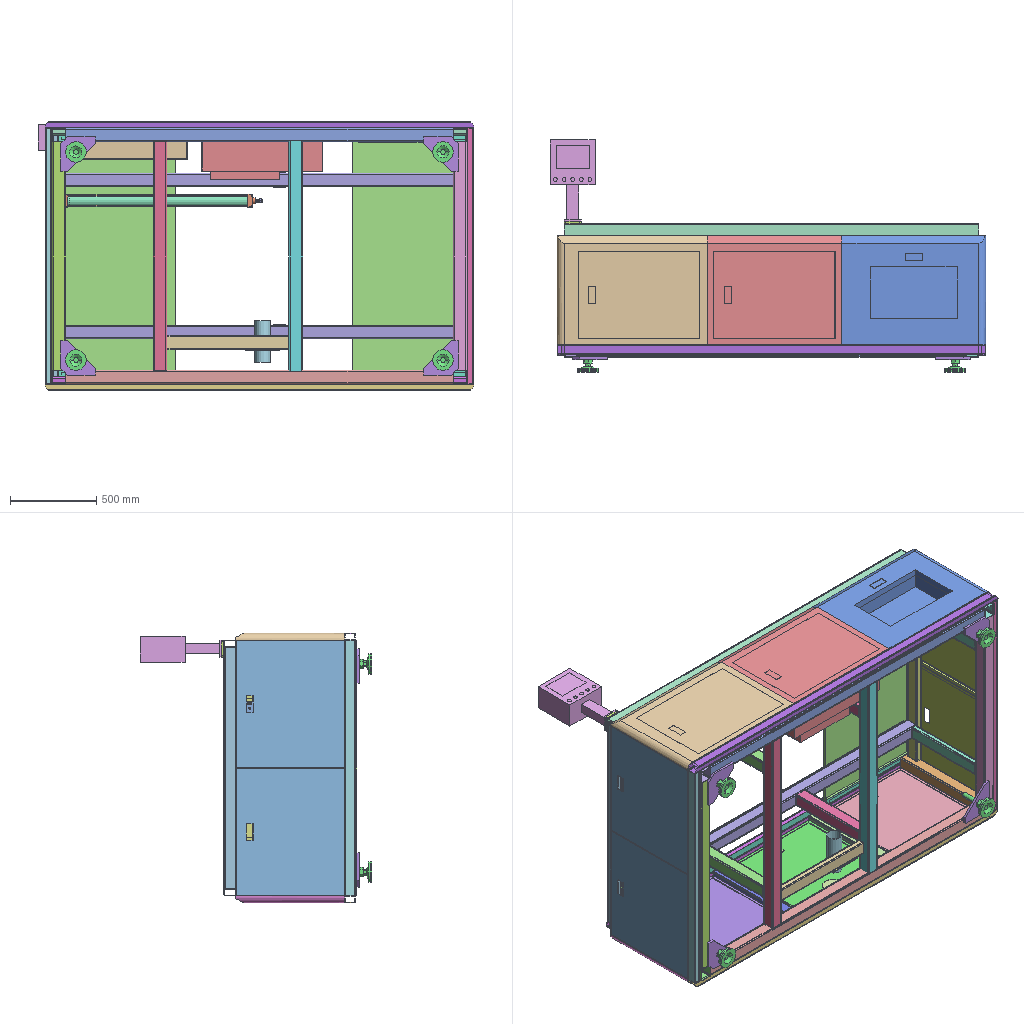Assembly | SolidWorks | 34 different items | 53 placed | box 2520 x 1341 x 1560 mm
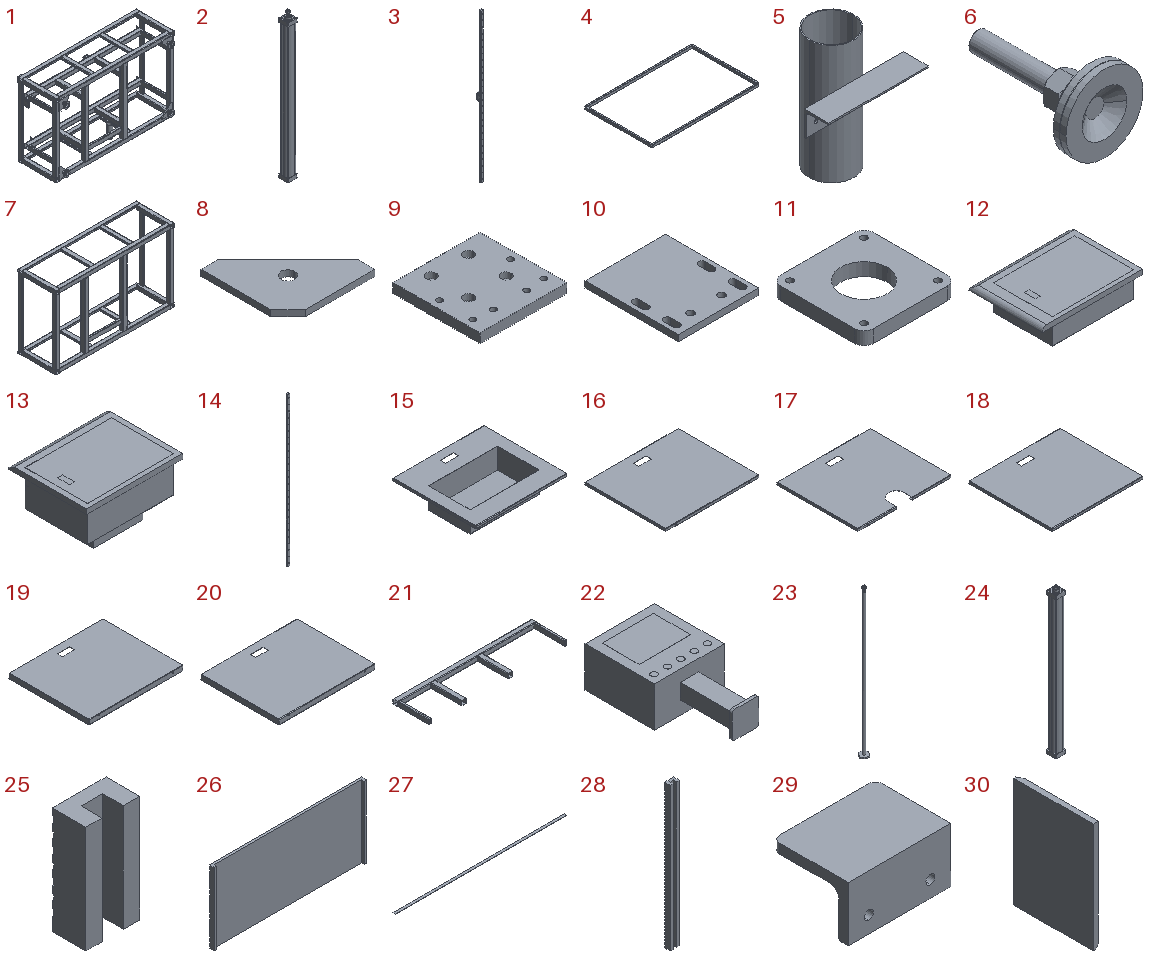Parts list (item | name | quantity | parent item | size | volume | features):
1 | (subassembly) | x1 | - | - | 41723102 mm3 | features ReferencePattern 2, CompositeCurve 1, LocalLPattern 1
2 | (subassembly) | x1 | - | 75 x 75 x 1153 mm | 1669537 mm3 | -
3 | (subassembly) | x2 | in 1 | 90 x 42.01 x 2080 mm | 1460108 mm3 | features LocalLPattern 1
4 | - | x1 | - | 2480 x 1560 x 60 mm | 4257292 mm3 | features 3DProfileFeature 1, ICE 1, WeldMemberFeat 1, WeldmentFeature 1
5 | - | x1 | in 1 | 200 x 140 x 240 mm | 210373 mm3 | features 3DProfileFeature 1, HoleWzd 1, ICE 1, WeldMemberFeat 1, WeldmentFeature 1
6 | - | x4 | in 1 | 120 x 197 x 120 mm | 378664 mm3 | features ICE 2, RevCut 2, Chamfer 1, Revolution 1
7 | - | x1 | in 1 | 2400 x 770 x 1480 mm | 23706901 mm3 | features WeldCornerFeat 5, WeldMemberFeat 4, 3DProfileFeature 2, WeldmentFeature 1
8 | - | x4 | in 1 | 200 x 200 x 14 mm | 358341 mm3 | features Extrusion 1
9 | - | x1 | in 1 | 130 x 130 x 14 mm | 224199 mm3 | features HoleWzd 3, Extrusion 1, ICE 1
10 | - | x1 | in 1 | 130 x 150 x 10 mm | 182698 mm3 | features HoleWzd 2, ICE 2, Extrusion 1
11 | - | x1 | in 1 | 100 x 100 x 14 mm | 109276 mm3 | features ICE 2, Extrusion 1, Fillet 1, HoleWzd 1
12 | - | x1 | - | 867.5 x 630 x 220 mm | 27389806 mm3 | features ICE 9, CutThin 1, Extrusion 1, Fillet 1, Shell 1
13 | - | x1 | - | 780 x 630 x 340 mm | 30091258 mm3 | features ICE 9, CutThin 1, Extrusion 1, Shell 1
14 | - | x2 | in 3 | 28 x 26 x 2080 mm | 1265174 mm3 | features ICE 19, MirrorPattern 5, Extrusion 4, MirrorSolid 4, Chamfer 3, Fillet 3, RevCut 3, Dome 2, LPattern 2, DeleteBody 1, LibraryFeature 1, Revolution 1
15 | - | x1 | - | 665 x 605 x 153.5 mm | 1290484 mm3 | features ICE 3, EdgeFlange 2, FlatPattern 1, SMBaseFlange 1, SheetMetal 1
16 | - | x1 | - | 700 x 605 x 20 mm | 761861 mm3 | features EdgeFlange 2, FlatPattern 1, HoleWzd 1, SMBaseFlange 1, SheetMetal 1
17 | - | x1 | - | 700 x 605 x 20 mm | 736343 mm3 | features EdgeFlange 2, FlatPattern 1, HoleWzd 1, ICE 1, SMBaseFlange 1, SheetMetal 1
18 | - | x1 | - | 665 x 605 x 20 mm | 726461 mm3 | features EdgeFlange 2, FlatPattern 1, HoleWzd 1, SMBaseFlange 1, SheetMetal 1
19 | - | x2 | - | 740 x 630 x 40 mm | 914335 mm3 | features EdgeFlange 2, FlatPattern 1, HoleWzd 1, SMBaseFlange 1, SheetMetal 1
20 | - | x2 | - | 740 x 600 x 40 mm | 876118 mm3 | features EdgeFlange 2, FlatPattern 1, HoleWzd 1, SMBaseFlange 1, SheetMetal 1
21 | - | x2 | in 1 | 2320 x 602 x 80 mm | 5618021 mm3 | features WeldMemberFeat 3, ICE 2, WeldCornerFeat 2, HoleWzd 1, LPattern 1, WeldmentFeature 1
22 | - | x1 | - | 260 x 470 x 150.5 mm | 11032431 mm3 | features ICE 3, Extrusion 1, Fillet 1
23 | - | x1 | in 2 | 63 x 63 x 1126 mm | 379367 mm3 | features ICE 5, Revolution 3, RevCut 2, Chamfer 1, Helix 1, LPattern 1, MirrorPattern 1, SweepCut 1
24 | - | x1 | in 2 | 75 x 75 x 1111 mm | 1290160 mm3 | features ICE 10, Fillet 4, Revolution 4, MirrorPattern 3, Chamfer 2, CirPattern 2, Helix 1, RevCut 1, SweepCut 1
25 | - | x2 | - | 80 x 50 x 160 mm | 470080 mm3 | features Extrusion 1, ICE 1, LPattern 1
26 | - | x2 | - | 1390 x 45 x 660 mm | 17341000 mm3 | features Extrusion 1, ICE 1, LPattern 1
27 | - | x2 | - | 2350 x 40 x 3 mm | 282000 mm3 | features Extrusion 1
28 | - | x2 | - | 72 x 45 x 1160 mm | 2864880 mm3 | features Extrusion 1, ICE 1, LPattern 1
29 | - | x4 | in 1 | 75 x 55 x 40 mm | 46347 mm3 | features 3DProfileFeature 1, Fillet 1, HoleWzd 1, ICE 1, WeldMemberFeat 1, WeldmentFeature 1
30 | - | x1 | - | 40 x 630 x 867.5 mm | 21184116 mm3 | features CutThin 1, Extrusion 1, Fillet 1
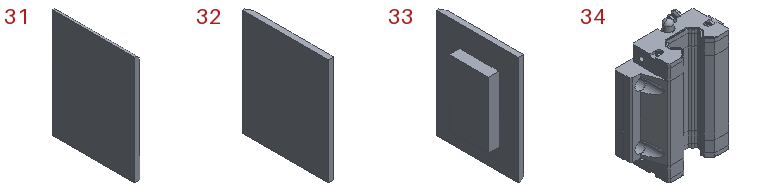31 | - | x1 | - | 40 x 630 x 832.5 mm | 20321060 mm3 | features CutThin 1, Extrusion 1, Fillet 1
32 | - | x1 | - | 40 x 630 x 780 mm | 19233148 mm3 | features CutThin 1, Extrusion 1
33 | - | x1 | - | 121.2 x 630 x 832.5 mm | 14657432 mm3 | features ICE 2, BossThin 1, CutThin 1, Extrusion 1, Fillet 1
34 | - | x2 | in 3 | 90 x 36.51 x 110.4 mm | 194935 mm3 | features ICE 23, Extrusion 5, MirrorPattern 5, Fillet 4, MirrorSolid 4, Chamfer 3, RevCut 3, Dome 2, LPattern 2, Revolution 2, DeleteBody 1, LibraryFeature 1
Mates (type | each side: item.copy, entity, surface, feature):
In the top assembly
Coincident | 7.1 face plane GB/6728-1986 square hollow section 080 X 80 X 4(1) | 15.1 face | 2 times
DistanceDim | 15.1 face | 7.1 face plane GB/6728-1986 rect hollow section 080 X 40 X 4(1)
Coincident | 7.1 face plane GB/6728-1986 square hollow section 080 X 80 X 4(1) | assembly face | 4 times
DistanceDim | assembly face | 7.1 face plane GB/6728-1986 square hollow section 080 X 80 X 4(1) | 2 times
Coincident | 7.1 face plane GB/6728-1986 square hollow section 080 X 80 X 4(1) | 16.1 face plane Base-Flange1
Coincident | 7.1 face plane GB/6728-1986 square hollow section 080 X 80 X 4(1) | 16.1 face plane Edge-Flange1
DistanceDim | 16.1 face plane Edge-Flange1 | 7.1 face plane GB/6728-1986 rect hollow section 080 X 40 X 4(1)
Coincident | 7.1 face plane GB/6728-1986 square hollow section 080 X 80 X 4(1) | 17.1 face plane Base-Flange1
DistanceDim | 17.1 face plane Edge-Flange1 | 7.1 face plane GB/6728-1986 rect hollow section 080 X 40 X 4(1)
Coincident | 7.1 face plane GB/6728-1986 square hollow section 080 X 80 X 4(1) | 17.1 face plane Edge-Flange1
Coincident | 7.1 face plane GB/6728-1986 square hollow section 080 X 80 X 4(1) | 18.1 face plane Edge-Flange1
Coincident | 7.1 face plane GB/6728-1986 square hollow section 080 X 80 X 4(1) | 18.1 face plane Base-Flange1
DistanceDim | 18.1 face plane Edge-Flange1 | 7.1 face plane GB/6728-1986 rect hollow section 080 X 40 X 4(1)
DistanceDim | 7.1 face plane GB/6728-1986 square hollow section 080 X 80 X 4(1) | 19.1 face plane Base-Flange1
Coincident | 19.1 face plane Base-Flange1 | 19.2 face plane Base-Flange1
DistanceDim | 7.1 face plane GB/6728-1986 square hollow section 080 X 80 X 4(1) | 20.1 face plane Base-Flange1
Coincident | 21.1 face plane Cut-Extrude1 | 25.1 face plane Boss-Extrude1
DistanceDim | 7.1 face plane GB/6728-1986 rect hollow section 080 X 40 X 4(1) | 25.1 face plane Boss-Extrude1
Width | 25.1 face plane Boss-Extrude1 | 25.1 face plane Boss-Extrude1 | assembly face
Coincident | 25.1 face plane Boss-Extrude1 | 25.2 face plane Boss-Extrude1 | 2 times
Width | 25.2 face plane Boss-Extrude1 | 25.2 face plane Boss-Extrude1 | assembly face
Coincident | 21.2 face plane Cut-Extrude1 | 28.1 face plane Boss-Extrude1
Coincident | 7.1 face plane GB/6728-1986 rect hollow section 080 X 40 X 4(1) | 28.1 face plane Boss-Extrude1
Width | 28.1 face plane Boss-Extrude1 | 28.1 face plane Boss-Extrude1 | assembly face
Width | 28.2 face plane Boss-Extrude1 | 28.2 face plane Boss-Extrude1 | assembly face
Coincident | 7.1 face plane GB/6728-1986 rect hollow section 080 X 40 X 4(1) | 28.2 face plane Boss-Extrude1
Coincident | 21.1 face plane Cut-Extrude1 | 28.2 face plane Boss-Extrude1
Coincident | 11.1 face plane Boss-Extrude1 | 22.1 face plane Boss-Extrude4 | 3 times
Coincident | 20.1 face plane Base-Flange1 | 20.2 face plane Base-Flange1
Coincident | 9.1 face plane Boss-Extrude1 | 24.1 face plane Boss-Extrude2
Concentric | 9.1 edge | 24.1 edge | 2 times
Width | 7.1 face plane GB/6728-1986 rect hollow section 080 X 40 X 4(1) | 7.1 face plane GB/6728-1986 rect hollow section 080 X 40 X 4(1) | 26.1 face plane Boss-Extrude1 | 26.1 face plane Boss-Extrude1
Width | 26.2 face plane Boss-Extrude1 | 26.2 face plane Boss-Extrude1 | 7.1 face plane GB/6728-1986 rect hollow section 080 X 40 X 4(1) | 7.1 face plane GB/6728-1986 rect hollow section 080 X 40 X 4(1)
Coincident | 7.1 face plane GB/6728-1986 square hollow section 080 X 80 X 4(1) | 26.2 face plane Boss-Extrude1
DistanceDim | 26.1 face plane Boss-Extrude1 | 7.1 face plane GB/6728-1986 rect hollow section 080 X 40 X 4(1)
DistanceDim | 7.1 face plane GB/6728-1986 square hollow section 080 X 80 X 4(1) | 4.1 face plane GB/6728-1986 rect hollow section 060 X 40 X 3(1)
Coincident | 7.1 face plane GB/6728-1986 square hollow section 080 X 80 X 4(1) | 4.1 face plane GB/6728-1986 rect hollow section 060 X 40 X 3(1) | 2 times
Coincident | 20.1 face plane Edge-Flange1 | 20.2 face plane Edge-Flange1
Width | 7.1 face plane GB/6728-1986 square hollow section 080 X 80 X 4(1) | 7.1 face plane GB/6728-1986 square hollow section 080 X 80 X 4(1) | 20.1 face plane Edge-Flange1 | 20.2 face plane Edge-Flange1
Coincident | 7.1 face plane GB/6728-1986 square hollow section 080 X 80 X 4(1) | 31.1 face plane Boss-Extrude1
Coincident | 20.2 face plane Base-Flange1 | 31.1 edge
Coincident | 19.1 face plane Edge-Flange1 | 19.2 face plane Edge-Flange1 | 2 times
Width | 7.1 face plane GB/6728-1986 square hollow section 080 X 80 X 4(1) | 7.1 face plane GB/6728-1986 square hollow section 080 X 80 X 4(1) | 19.2 face plane Edge-Flange1 | 19.1 face plane Edge-Flange1
Coincident | 20.1 face plane Edge-Flange1 | 4.1 face plane GB/6728-1986 rect hollow section 060 X 40 X 3(1)
Coincident | 20.2 face plane Edge-Flange1 | 4.1 face plane GB/6728-1986 rect hollow section 060 X 40 X 3(1)
Coincident | 4.1 face plane GB/6728-1986 rect hollow section 060 X 40 X 3(1) | 31.1 face plane Boss-Extrude1
Coincident | 19.1 face plane Edge-Flange1 | 4.1 face plane GB/6728-1986 rect hollow section 060 X 40 X 3(1)
Coincident | 7.1 face plane GB/6728-1986 square hollow section 080 X 80 X 4(1) | 12.1 face plane Boss-Extrude7
Coincident | 12.1 face plane Boss-Extrude7 | 4.1 face plane GB/6728-1986 rect hollow section 060 X 40 X 3(1)
Coincident | 7.1 face plane GB/6728-1986 rect hollow section 080 X 40 X 4(1) | 13.1 face plane Boss-Extrude7
Coincident | 4.1 face plane GB/6728-1986 rect hollow section 060 X 40 X 3(1) | 13.1 face plane Boss-Extrude7
Coincident | 12.1 edge | 4.1 face plane GB/6728-1986 rect hollow section 060 X 40 X 3(1)
DistanceDim | 13.1 face plane Boss-Extrude1 | 7.1 face plane GB/6728-1986 rect hollow section 080 X 40 X 4(1)
Coincident | 4.1 face plane GB/6728-1986 rect hollow section 060 X 40 X 3(1) | 33.1 face plane Boss-Extrude1
Coincident | 7.1 face plane GB/6728-1986 square hollow section 080 X 80 X 4(1) | 33.1 face plane Boss-Extrude1
Coincident | 13.1 face plane Boss-Extrude7 | 33.1 face plane Boss-Extrude1
Coincident | 31.1 face plane Boss-Extrude1 | 32.1 face plane Boss-Extrude1
Coincident | 7.1 face plane GB/6728-1986 rect hollow section 080 X 40 X 4(1) | 32.1 face plane Boss-Extrude1
Coincident | 4.1 face plane GB/6728-1986 rect hollow section 060 X 40 X 3(1) | 32.1 face plane Boss-Extrude1
Coincident | 7.1 face plane GB/6728-1986 square hollow section 080 X 80 X 4(1) | 30.1 face plane Boss-Extrude1
Coincident | 4.1 face plane GB/6728-1986 rect hollow section 060 X 40 X 3(1) | 30.1 face plane Boss-Extrude1
Coincident | 32.1 face plane Boss-Extrude1 | 30.1 face plane Boss-Extrude1
Coincident | 7.1 face plane GB/6728-1986 square hollow section 080 X 80 X 4(1) | 27.1 face plane Boss-Extrude1
Coincident | 7.1 face plane GB/6728-1986 rect hollow section 080 X 40 X 4(1) | 27.1 face plane Boss-Extrude1 | 2 times
Coincident | 7.1 face plane GB/6728-1986 rect hollow section 080 X 40 X 4(1) | 27.2 face plane Boss-Extrude1 | 2 times
Coincident | 7.1 face plane GB/6728-1986 square hollow section 080 X 80 X 4(1) | 27.2 face plane Boss-Extrude1
Coincident | 26.2 face plane Boss-Extrude1 | 27.1 face plane Boss-Extrude1
In subassembly 1
Coincident | 7.2 face plane GB/6728-1986 square hollow section 080 X 80 X 4(1) | 8.1 face plane Boss-Extrude1
DistanceDim | 8.1 face plane Boss-Extrude1 | 7.2 face plane GB/6728-1986 square hollow section 080 X 80 X 4(1) | 2 times
Coincident | 7.2 face plane GB/6728-1986 square hollow section 080 X 80 X 4(1) | 8.2 face plane Boss-Extrude1
DistanceDim | 8.2 face plane Boss-Extrude1 | 7.2 face plane GB/6728-1986 square hollow section 080 X 80 X 4(1) | 2 times
Coincident | 7.2 face plane GB/6728-1986 square hollow section 080 X 80 X 4(1) | 8.3 face plane Boss-Extrude1
DistanceDim | 7.2 face plane GB/6728-1986 square hollow section 080 X 80 X 4(1) | 8.3 face plane Boss-Extrude1
DistanceDim | 8.3 face plane Boss-Extrude1 | 7.2 face plane GB/6728-1986 square hollow section 080 X 80 X 4(1)
Coincident | 7.2 face plane GB/6728-1986 square hollow section 080 X 80 X 4(1) | 8.4 face plane Boss-Extrude1
DistanceDim | 8.4 face plane Boss-Extrude1 | 7.2 face plane GB/6728-1986 square hollow section 080 X 80 X 4(1)
DistanceDim | 7.2 face plane GB/6728-1986 square hollow section 080 X 80 X 4(1) | 8.4 face plane Boss-Extrude1
Concentric | 6.1 face cylinder Revolve1 | 8.2 face cylinder Boss-Extrude1
Coincident | 6.1 face plane Boss-Extrude2 | 8.2 face plane Boss-Extrude1
Coincident | 8.3 face plane Boss-Extrude1 | 6.2 face plane Boss-Extrude2
Concentric | 8.3 face cylinder Boss-Extrude1 | 6.2 face cylinder Revolve1
Coincident | 8.4 face plane Boss-Extrude1 | 6.3 face plane Boss-Extrude2
Concentric | 8.4 face cylinder Boss-Extrude1 | 6.3 face cylinder Revolve1
Coincident | 8.1 face plane Boss-Extrude1 | 6.4 face plane Boss-Extrude2
Concentric | 8.1 face cylinder Boss-Extrude1 | 6.4 face cylinder Revolve1
Coincident | 9.2 face plane Boss-Extrude1 | 10.1 face plane Boss-Extrude1
Concentric | 9.2 face cylinder M10 Tapped Hole1 | 10.1 face cylinder Ø11.0 (11) Diameter Hole1 | 2 times
Coincident | 1.1 face | 1.1 face | 2 times
Coincident | 7.2 face plane GB/6728-1986 square hollow section 080 X 80 X 4(1) | 21.3 face plane GB/6728-1986 rect hollow section 080 X 40 X 4(1)
Coincident | 7.2 face plane GB/6728-1986 rect hollow section 080 X 40 X 4(1) | 21.3 face plane GB/6728-1986 rect hollow section 080 X 40 X 4(1)
Coincident | 21.3 face plane GB/6728-1986 square hollow section 080 X 80 X 4(1) | 21.4 face plane GB/6728-1986 square hollow section 080 X 80 X 4(1)
Coincident | 21.3 face plane GB/6728-1986 rect hollow section 080 X 40 X 4(1) | 21.4 face plane GB/6728-1986 rect hollow section 080 X 40 X 4(1)
DistanceDim | 21.3 face plane GB/6728-1986 square hollow section 080 X 80 X 4(1) | 21.4 face plane GB/6728-1986 square hollow section 080 X 80 X 4(1)
Width | 7.2 face plane GB/6728-1986 rect hollow section 080 X 40 X 4(1) | 7.2 face plane GB/6728-1986 rect hollow section 080 X 40 X 4(1) | 21.3 face plane GB/6728-1986 square hollow section 080 X 80 X 4(1) | 21.4 face plane GB/6728-1986 square hollow section 080 X 80 X 4(1)
Coincident | 1.1 face | 21.4 face plane GB/6728-1986 square hollow section 080 X 80 X 4(1)
Width | 21.4 face plane GB/6728-1986 square hollow section 080 X 80 X 4(1) | 21.4 face plane GB/6728-1986 square hollow section 080 X 80 X 4(1) | 1.1 face
Coincident | 7.2 face plane GB/6728-1986 rect hollow section 080 X 40 X 4(1) | 11.2 face plane Boss-Extrude1 | 3 times
Coincident | 7.2 face plane GB/6728-1986 rect hollow section 080 X 40 X 4(1) | 10.1 face plane Boss-Extrude1
DistanceDim | 10.1 face plane Boss-Extrude2 | 7.2 face plane GB/6728-1986 rect hollow section 080 X 40 X 4(1)
DistanceDim | 9.2 face plane Boss-Extrude1 | 7.2 face plane GB/6728-1986 rect hollow section 080 X 40 X 4(1)
Coincident | 7.2 face plane GB/6728-1986 rect hollow section 080 X 40 X 3(1) | 5.1 face plane Equal angle 5X4(1) | 2 times
Width | 7.2 face plane GB/6728-1986 rect hollow section 080 X 40 X 4(1) | 7.2 face plane GB/6728-1986 rect hollow section 080 X 40 X 4(1) | 5.1 face cylinder Boss-Extrude1
Coincident | 7.2 face plane GB/6728-1986 rect hollow section 080 X 40 X 4(1) | 29.1 face plane Unequal angle 6.3-4(1)
Width | 29.1 face plane Unequal angle 6.3-4(1) | 29.1 face plane Unequal angle 6.3-4(1) | 21.4 face plane GB/6728-1986 square hollow section 080 X 80 X 4(1) | 21.4 face plane GB/6728-1986 square hollow section 080 X 80 X 4(1)
Coincident | 21.4 face plane Cut-Extrude1 | 29.2 face plane Unequal angle 6.3-4(1)
Coincident | 29.1 face plane Unequal angle 6.3-4(1) | 29.2 face plane Unequal angle 6.3-4(1)
Coincident | 21.4 face plane Cut-Extrude1 | 14.1 face plane Boss-Extrude10
Concentric | 21.4 face cylinder M8 Tapped Hole1 | 14.1 face cylinder Cut-Revolve2
Parallel | 21.4 face plane GB/6728-1986 square hollow section 080 X 80 X 4(1) | 14.1 face plane Boss-Extrude10
Coincident | 21.3 face plane Cut-Extrude1 | 14.2 face plane Boss-Extrude10
Concentric | 21.3 face cylinder M8 Tapped Hole1 | 14.2 face cylinder Cut-Revolve2
Parallel | 21.3 face plane GB/6728-1986 square hollow section 080 X 80 X 4(1) | 14.2 face plane Boss-Extrude10
In subassembly 3
Coincident | 34.1 face plane Cut-Extrude11 | 14.3 face plane Boss-Extrude10 | 2 times
Path | 34.1 select_type:25 | 14.3 select_type:0
In subassembly 2
Concentric | 24.2 face cylinder Revolve2 | 23.1 face cylinder Revolve1
Coincident | 24.2 face plane Boss-Extrude2 | 23.1 face plane Revolve1